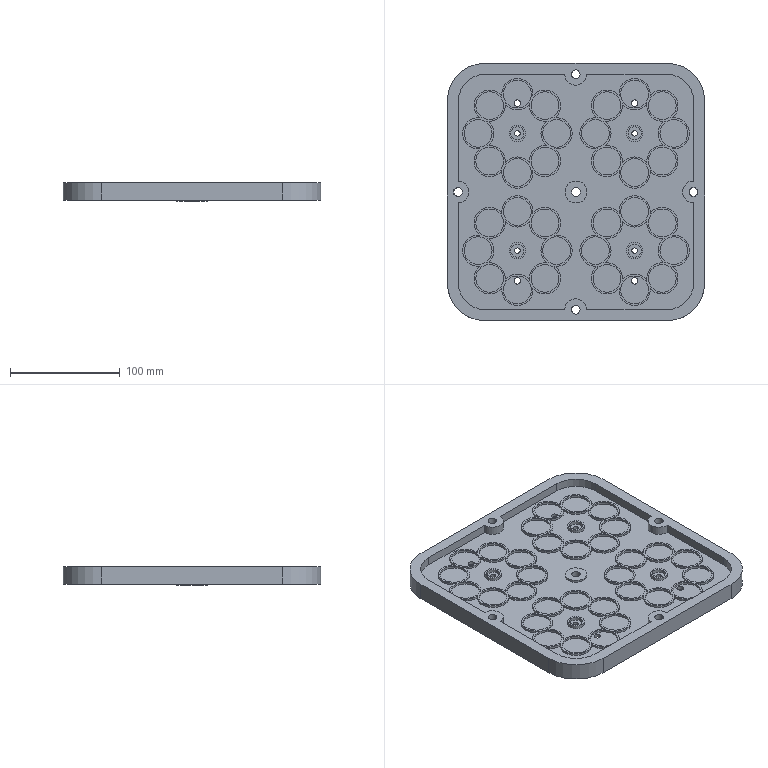Part | SolidWorks | features ICE 7, Extrusion 1 | 1 solid | 385 faces | box 235 x 235 x 17 mm | volume 295331 mm3 | cylinder 290 | plane 95 | commonest cylinder face diameters 28.5 x104 25.4 x64 20 x28 8 x18 15 x16 43 x12